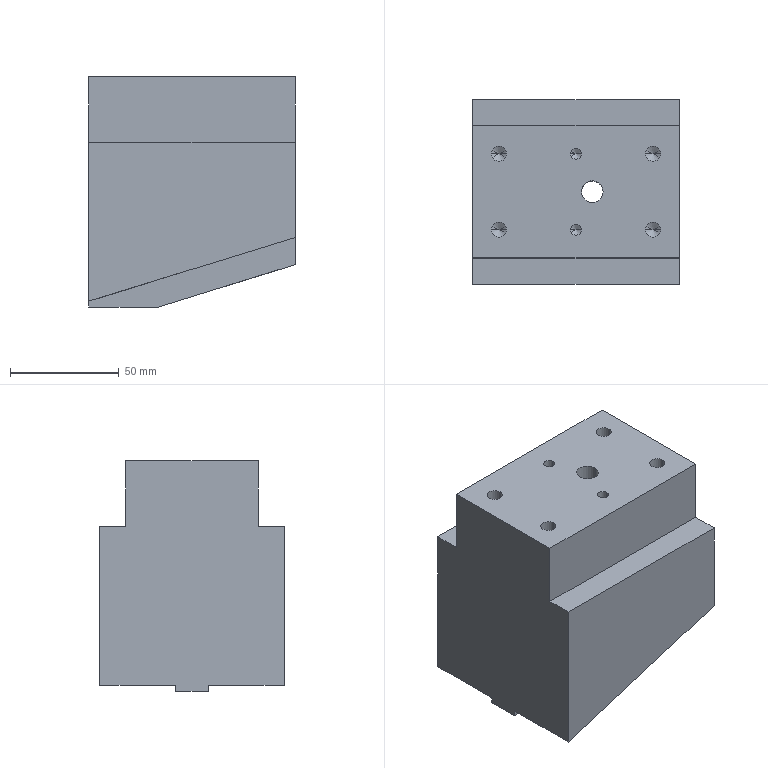Part | 1 solid | 61 faces | box 95 x 85 x 106 mm | volume 594913 mm3 | plane 25 | cylinder 20 | cone 12 | spline 4 | commonest cylinder face diameters 7 x8 25 x6 5 x4 10 x2